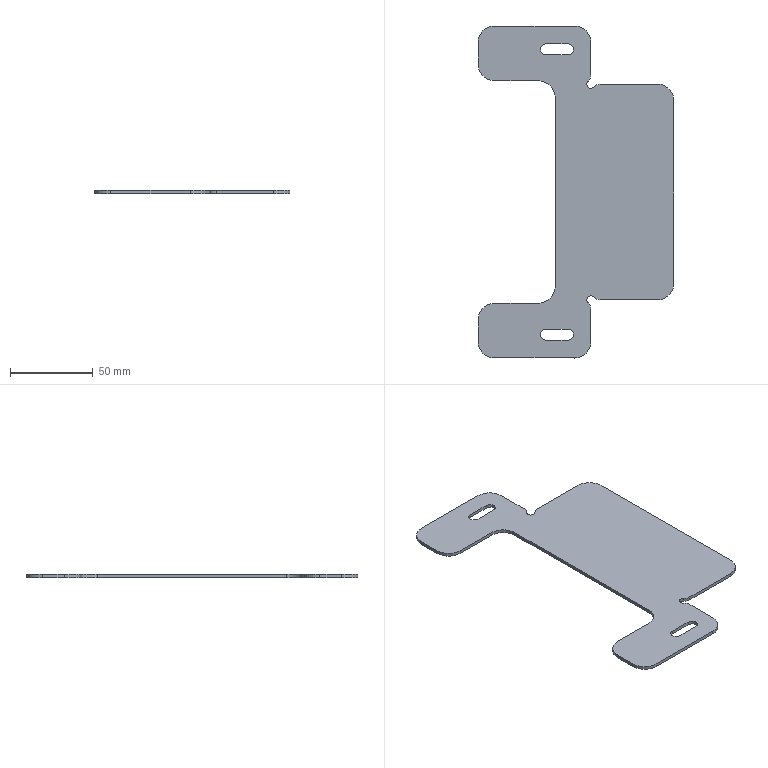Part | STEP file | 冲床-300配套压波_id578_x_t | 1 solid | 38 faces | box 118 x 200 x 2 mm | volume 26939 mm3 | plane 18 | cylinder 14 | spline 6 | commonest cylinder face diameters 20 x10 6.5 x4